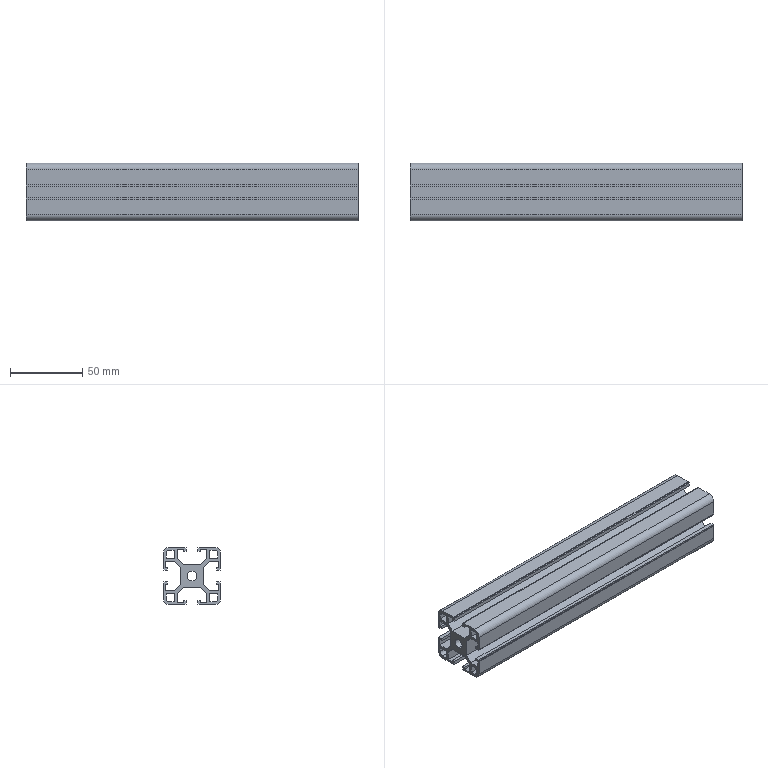Part | SolidWorks | features WeldMemberFeat 1, WeldmentFeature 1 | 1 solid | 104 faces | box 230 x 40 x 40 mm | volume 132605 mm3 | plane 94 | cylinder 10 | commonest cylinder face diameters 5 x4 9 x4 6.8 x2